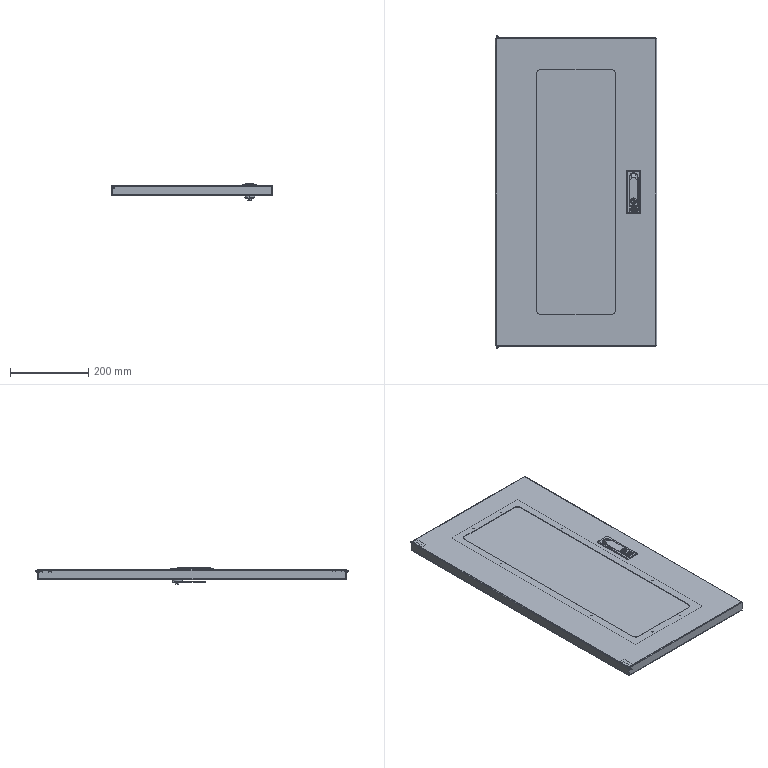Part | SolidWorks | 7 solids | 476 faces | box 411 x 799 x 42.5 mm | volume 1154283 mm3 | plane 256 | cylinder 180 | spline 28 | cone 12 | commonest cylinder face diameters 4 x50 3 x21 1 x17 2 x15 12 x8 8 x6